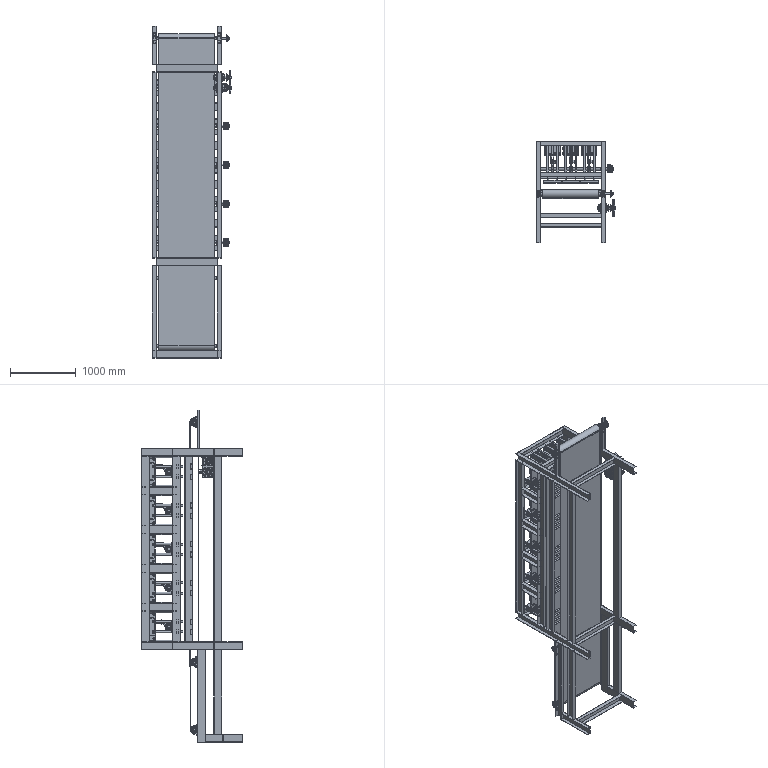Part | SolidWorks | features ReferencePattern 140, InContextFeatHolder 10, LocalLPattern 2, LocalSketchPattern 2, MirrorCompFeat 2 | 1127 solids | 41936 faces | volume 264532636 mm3 | cylinder 18356 | plane 17252 | cone 3072 | torus 2850 | sphere 328 | spline 78 | commonest cylinder face diameters 6.5 x3600 22.1 x1320 35.1 x1320 14.747 x968 26.567 x968 40 x763